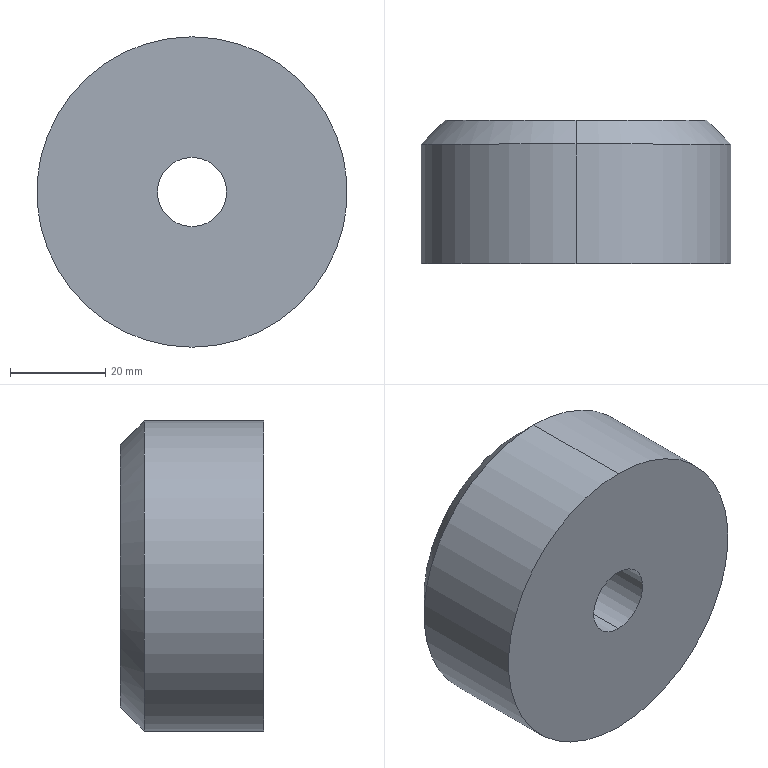Part | SolidWorks | features Chamfer 1, Extrusion 1, HoleWzd 1 | 1 solid | 8 faces | box 65 x 30 x 65 mm | volume 92174 mm3 | cylinder 4 | cone 2 | plane 2 | commonest cylinder face diameters 14.5 x2 65 x2
STEP:
#1=CARTESIAN_POINT('',(0.,0.,-7.25));
#2=VERTEX_POINT('',#1);
#3=CARTESIAN_POINT('',(0.,0.,7.25));
#4=VERTEX_POINT('',#3);
#5=CARTESIAN_POINT('',(0.,0.,0.));
#6=DIRECTION('',(0.,1.,0.));
#7=DIRECTION('',(0.,0.,1.));
#8=AXIS2_PLACEMENT_3D('',#5,#6,#7);
#9=CIRCLE('',#8,7.25);
#10=EDGE_CURVE('',#2,#4,#9,.T.);
#11=ORIENTED_EDGE('',*,*,#10,.F.);
#12=CARTESIAN_POINT('',(0.,30.,-7.25));
#13=VERTEX_POINT('',#12);
#14=CARTESIAN_POINT('',(0.,30.,-7.25));
#15=DIRECTION('',(0.,1.,0.));
#16=VECTOR('',#15,1000.);
#17=LINE('',#14,#16);
#18=EDGE_CURVE('',#2,#13,#17,.T.);
#19=ORIENTED_EDGE('',*,*,#18,.T.);
#20=CARTESIAN_POINT('',(0.,30.,7.25));
#21=VERTEX_POINT('',#20);
#22=CARTESIAN_POINT('',(0.,30.,0.));
#23=DIRECTION('',(0.,1.,0.));
#24=DIRECTION('',(0.,0.,1.));
#25=AXIS2_PLACEMENT_3D('',#22,#23,#24);
#26=CIRCLE('',#25,7.25);
#27=EDGE_CURVE('',#13,#21,#26,.T.);
#28=ORIENTED_EDGE('',*,*,#27,.T.);
#29=CARTESIAN_POINT('',(0.,30.,7.25));
#30=DIRECTION('',(0.,1.,0.));
#31=VECTOR('',#30,1000.);
#32=LINE('',#29,#31);
#33=EDGE_CURVE('',#4,#21,#32,.T.);
#34=ORIENTED_EDGE('',*,*,#33,.F.);
#35=EDGE_LOOP('',(#11,#19,#28,#34));
#36=FACE_OUTER_BOUND('',#35,.T.);
#37=CARTESIAN_POINT('',(0.,30.,0.));
#38=DIRECTION('',(0.,1.,0.));
#39=DIRECTION('',(0.,0.,1.));
#40=AXIS2_PLACEMENT_3D('',#37,#38,#39);
#41=CYLINDRICAL_SURFACE('',#40,7.25);
#42=ADVANCED_FACE('',(#36),#41,.F.);
#43=CARTESIAN_POINT('',(0.,30.,27.5));
#44=VERTEX_POINT('',#43);
#45=CARTESIAN_POINT('',(0.,30.,-27.5));
#46=VERTEX_POINT('',#45);
#47=CARTESIAN_POINT('',(0.,30.,0.));
#48=DIRECTION('',(0.,1.,0.));
#49=DIRECTION('',(0.,0.,1.));
#50=AXIS2_PLACEMENT_3D('',#47,#48,#49);
#51=CIRCLE('',#50,27.5);
#52=EDGE_CURVE('',#44,#46,#51,.T.);
#53=ORIENTED_EDGE('',*,*,#52,.F.);
#54=CARTESIAN_POINT('',(0.,25.,32.5));
#55=VERTEX_POINT('',#54);
#56=CARTESIAN_POINT('',(0.,30.,27.5));
#57=DIRECTION('',(0.,-0.7071,0.7071));
#58=VECTOR('',#57,1000.);
#59=LINE('',#56,#58);
#60=EDGE_CURVE('',#44,#55,#59,.T.);
#61=ORIENTED_EDGE('',*,*,#60,.T.);
#62=CARTESIAN_POINT('',(0.,25.,-32.5));
#63=VERTEX_POINT('',#62);
#64=CARTESIAN_POINT('',(0.,25.,0.));
#65=DIRECTION('',(0.,-1.,0.));
#66=DIRECTION('',(0.,0.,1.));
#67=AXIS2_PLACEMENT_3D('',#64,#65,#66);
#68=CIRCLE('',#67,32.5);
#69=EDGE_CURVE('',#63,#55,#68,.T.);
#70=ORIENTED_EDGE('',*,*,#69,.F.);
#71=CARTESIAN_POINT('',(0.,30.,-27.5));
#72=DIRECTION('',(0.,-0.7071,-0.7071));
#73=VECTOR('',#72,1000.);
#74=LINE('',#71,#73);
#75=EDGE_CURVE('',#46,#63,#74,.T.);
#76=ORIENTED_EDGE('',*,*,#75,.F.);
#77=EDGE_LOOP('',(#53,#61,#70,#76));
#78=FACE_OUTER_BOUND('',#77,.T.);
#79=CARTESIAN_POINT('',(0.,30.,0.));
#80=DIRECTION('',(0.,-1.,0.));
#81=DIRECTION('',(0.,0.,-1.));
#82=AXIS2_PLACEMENT_3D('',#79,#80,#81);
#83=CONICAL_SURFACE('',#82,27.5,0.7854);
#84=ADVANCED_FACE('',(#78),#83,.T.);
#85=ORIENTED_EDGE('',*,*,#69,.T.);
#86=CARTESIAN_POINT('',(0.,0.,32.5));
#87=VERTEX_POINT('',#86);
#88=CARTESIAN_POINT('',(0.,30.,32.5));
#89=DIRECTION('',(0.,-1.,0.));
#90=VECTOR('',#89,1000.);
#91=LINE('',#88,#90);
#92=EDGE_CURVE('',#55,#87,#91,.T.);
#93=ORIENTED_EDGE('',*,*,#92,.T.);
#94=CARTESIAN_POINT('',(0.,0.,-32.5));
#95=VERTEX_POINT('',#94);
#96=CARTESIAN_POINT('',(0.,0.,0.));
#97=DIRECTION('',(0.,1.,0.));
#98=DIRECTION('',(0.,0.,1.));
#99=AXIS2_PLACEMENT_3D('',#96,#97,#98);
#100=CIRCLE('',#99,32.5);
#101=EDGE_CURVE('',#87,#95,#100,.T.);
#102=ORIENTED_EDGE('',*,*,#101,.T.);
#103=CARTESIAN_POINT('',(0.,30.,-32.5));
#104=DIRECTION('',(0.,-1.,0.));
#105=VECTOR('',#104,1000.);
#106=LINE('',#103,#105);
#107=EDGE_CURVE('',#63,#95,#106,.T.);
#108=ORIENTED_EDGE('',*,*,#107,.F.);
#109=EDGE_LOOP('',(#85,#93,#102,#108));
#110=FACE_OUTER_BOUND('',#109,.T.);
#111=CARTESIAN_POINT('',(0.,30.,0.));
#112=DIRECTION('',(0.,-1.,0.));
#113=DIRECTION('',(0.,0.,-1.));
#114=AXIS2_PLACEMENT_3D('',#111,#112,#113);
#115=CYLINDRICAL_SURFACE('',#114,32.5);
#116=ADVANCED_FACE('',(#110),#115,.T.);
#117=ORIENTED_EDGE('',*,*,#92,.F.);
#118=CARTESIAN_POINT('',(0.,25.,0.));
#119=DIRECTION('',(0.,-1.,0.));
#120=DIRECTION('',(0.,0.,1.));
#121=AXIS2_PLACEMENT_3D('',#118,#119,#120);
#122=CIRCLE('',#121,32.5);
#123=EDGE_CURVE('',#55,#63,#122,.T.);
#124=ORIENTED_EDGE('',*,*,#123,.T.);
#125=ORIENTED_EDGE('',*,*,#107,.T.);
#126=CARTESIAN_POINT('',(0.,0.,0.));
#127=DIRECTION('',(0.,1.,0.));
#128=DIRECTION('',(0.,0.,1.));
#129=AXIS2_PLACEMENT_3D('',#126,#127,#128);
#130=CIRCLE('',#129,32.5);
#131=EDGE_CURVE('',#95,#87,#130,.T.);
#132=ORIENTED_EDGE('',*,*,#131,.T.);
#133=EDGE_LOOP('',(#117,#124,#125,#132));
#134=FACE_OUTER_BOUND('',#133,.T.);
#135=CARTESIAN_POINT('',(0.,30.,0.));
#136=DIRECTION('',(0.,-1.,0.));
#137=DIRECTION('',(0.,0.,-1.));
#138=AXIS2_PLACEMENT_3D('',#135,#136,#137);
#139=CYLINDRICAL_SURFACE('',#138,32.5);
#140=ADVANCED_FACE('',(#134),#139,.T.);
#141=CARTESIAN_POINT('',(0.,30.,0.));
#142=DIRECTION('',(0.,1.,0.));
#143=DIRECTION('',(0.,0.,1.));
#144=AXIS2_PLACEMENT_3D('',#141,#142,#143);
#145=CIRCLE('',#144,7.25);
#146=EDGE_CURVE('',#21,#13,#145,.T.);
#147=ORIENTED_EDGE('',*,*,#146,.F.);
#148=ORIENTED_EDGE('',*,*,#27,.F.);
#149=EDGE_LOOP('',(#147,#148));
#150=FACE_BOUND('',#149,.T.);
#151=CARTESIAN_POINT('',(0.,30.,0.));
#152=DIRECTION('',(0.,1.,0.));
#153=DIRECTION('',(0.,0.,1.));
#154=AXIS2_PLACEMENT_3D('',#151,#152,#153);
#155=CIRCLE('',#154,27.5);
#156=EDGE_CURVE('',#46,#44,#155,.T.);
#157=ORIENTED_EDGE('',*,*,#156,.T.);
#158=ORIENTED_EDGE('',*,*,#52,.T.);
#159=EDGE_LOOP('',(#157,#158));
#160=FACE_OUTER_BOUND('',#159,.T.);
#161=CARTESIAN_POINT('',(0.,30.,0.));
#162=DIRECTION('',(0.,1.,0.));
#163=DIRECTION('',(0.,0.,1.));
#164=AXIS2_PLACEMENT_3D('',#161,#162,#163);
#165=PLANE('',#164);
#166=ADVANCED_FACE('',(#150,#160),#165,.T.);
#167=CARTESIAN_POINT('',(0.,0.,0.));
#168=DIRECTION('',(0.,1.,0.));
#169=DIRECTION('',(0.,0.,1.));
#170=AXIS2_PLACEMENT_3D('',#167,#168,#169);
#171=CIRCLE('',#170,7.25);
#172=EDGE_CURVE('',#4,#2,#171,.T.);
#173=ORIENTED_EDGE('',*,*,#172,.T.);
#174=ORIENTED_EDGE('',*,*,#10,.T.);
#175=EDGE_LOOP('',(#173,#174));
#176=FACE_BOUND('',#175,.T.);
#177=ORIENTED_EDGE('',*,*,#131,.F.);
#178=ORIENTED_EDGE('',*,*,#101,.F.);
#179=EDGE_LOOP('',(#177,#178));
#180=FACE_OUTER_BOUND('',#179,.T.);
#181=CARTESIAN_POINT('',(0.,0.,0.));
#182=DIRECTION('',(0.,1.,0.));
#183=DIRECTION('',(0.,0.,1.));
#184=AXIS2_PLACEMENT_3D('',#181,#182,#183);
#185=PLANE('',#184);
#186=ADVANCED_FACE('',(#176,#180),#185,.F.);
#187=ORIENTED_EDGE('',*,*,#60,.F.);
#188=ORIENTED_EDGE('',*,*,#156,.F.);
#189=ORIENTED_EDGE('',*,*,#75,.T.);
#190=ORIENTED_EDGE('',*,*,#123,.F.);
#191=EDGE_LOOP('',(#187,#188,#189,#190));
#192=FACE_OUTER_BOUND('',#191,.T.);
#193=CARTESIAN_POINT('',(0.,30.,0.));
#194=DIRECTION('',(0.,-1.,0.));
#195=DIRECTION('',(0.,0.,-1.));
#196=AXIS2_PLACEMENT_3D('',#193,#194,#195);
#197=CONICAL_SURFACE('',#196,27.5,0.7854);
#198=ADVANCED_FACE('',(#192),#197,.T.);
#199=ORIENTED_EDGE('',*,*,#18,.F.);
#200=ORIENTED_EDGE('',*,*,#172,.F.);
#201=ORIENTED_EDGE('',*,*,#33,.T.);
#202=ORIENTED_EDGE('',*,*,#146,.T.);
#203=EDGE_LOOP('',(#199,#200,#201,#202));
#204=FACE_OUTER_BOUND('',#203,.T.);
#205=CARTESIAN_POINT('',(0.,30.,0.));
#206=DIRECTION('',(0.,1.,0.));
#207=DIRECTION('',(0.,0.,1.));
#208=AXIS2_PLACEMENT_3D('',#205,#206,#207);
#209=CYLINDRICAL_SURFACE('',#208,7.25);
#210=ADVANCED_FACE('',(#204),#209,.F.);
#211=CLOSED_SHELL('',(#42,#84,#116,#140,#166,#186,#198,#210));
#212=MANIFOLD_SOLID_BREP('',#211);
#213=CARTESIAN_POINT('',(0.,0.,0.));
#214=DIRECTION('',(0.,0.,1.));
#215=DIRECTION('',(1.,0.,0.));
#216=AXIS2_PLACEMENT_3D('',#213,#214,#215);
#217=(LENGTH_UNIT()NAMED_UNIT(*)SI_UNIT(.MILLI.,.METRE.));
#218=UNCERTAINTY_MEASURE_WITH_UNIT(LENGTH_MEASURE(0.00001),#217,'','');
#219=(NAMED_UNIT(*)PLANE_ANGLE_UNIT()SI_UNIT($,.RADIAN.));
#220=(NAMED_UNIT(*)SI_UNIT($,.STERADIAN.)SOLID_ANGLE_UNIT());
#221=(GEOMETRIC_REPRESENTATION_CONTEXT(3)GLOBAL_UNCERTAINTY_ASSIGNED_CONTEXT((#218))GLOBAL_UNIT_ASSIGNED_CONTEXT((#217,#219,#220))REPRESENTATION_CONTEXT('',''));
#222=ADVANCED_BREP_SHAPE_REPRESENTATION('',(#212,#216),#221);